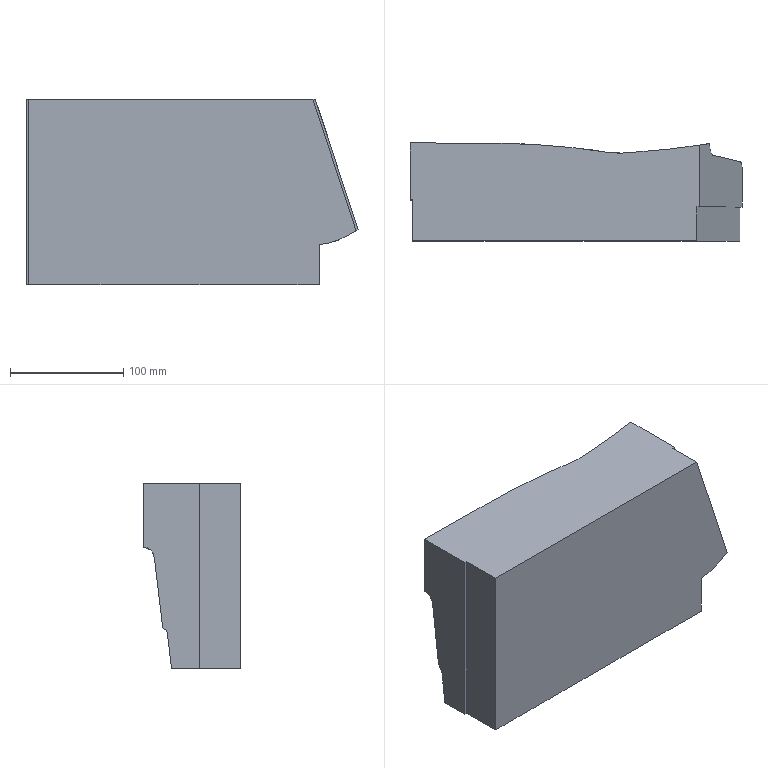Part | NX | features solid 2 | 1 solid | 64 faces | box 293.06 x 86.432 x 164.005 mm | volume 3103934 mm3 | spline 55 | plane 9